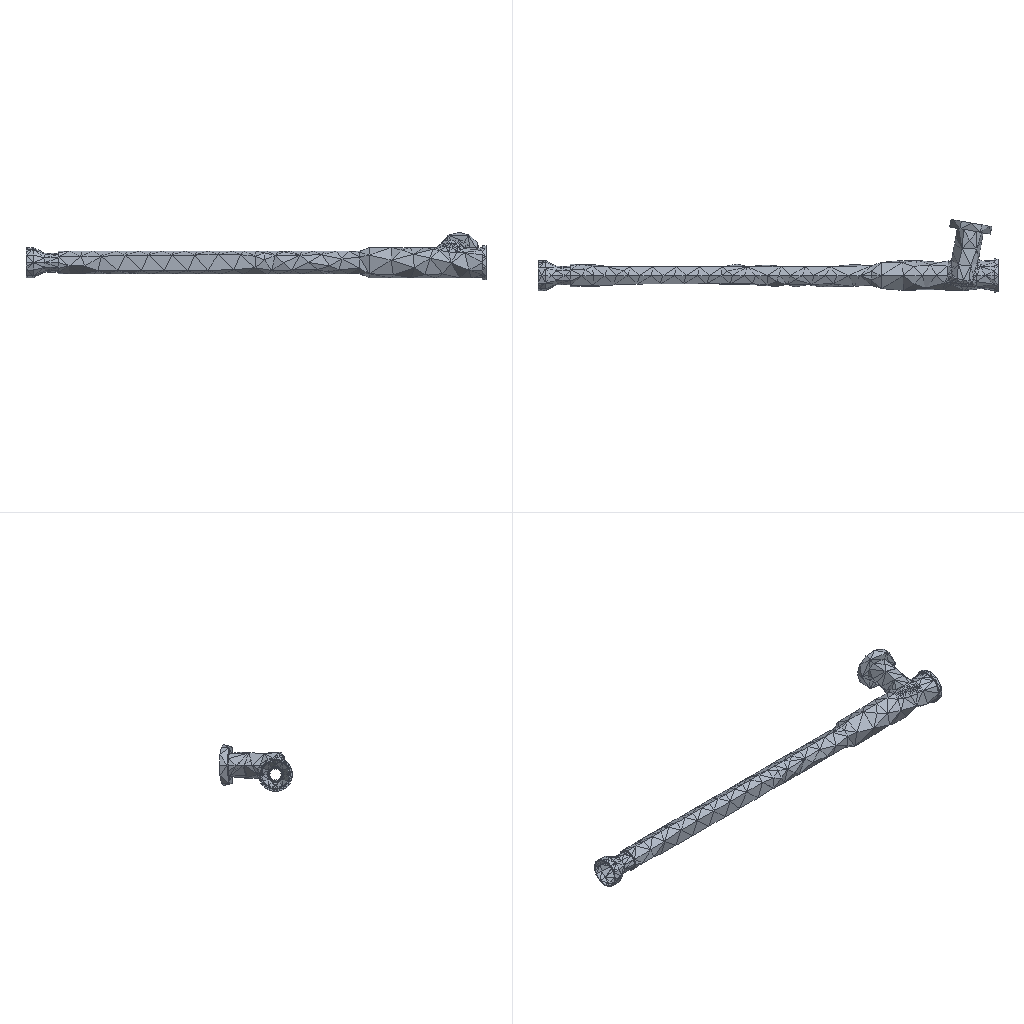Simulation study | ansys workbench
Ansys APDL input file, long lists of numbers shortened:
/batch
/config,noeldb,1     ! force off writing results to database
*get,_wallstrt,active,,time,wall
! ANSYS input file written by Workbench version 2022 R1
! File used for geometry attach: F:\ansys（分析文件汇总)\ansys转向器有限元分析\转向器\分析\动力缸体.STEP
/title,wbnew--____ (H5)
! ****** Begin Custom Load Command Snippet ******
/COM, ACT Extensions:
/COM,     LSDYNA, 2021.1
/COM,
! ****** End   Custom Load Command Snippet ******
*DIM,_wb_ProjectScratch_dir,string,248
_wb_ProjectScratch_dir(1) = 'C:\Users\Administrator\AppData\Local\Temp\WB_Administrator_18756_2\_ProjectScratch\Scr1D13\'
*DIM,_wb_SolverFiles_dir,string,248
_wb_SolverFiles_dir(1) = 'C:\Users\Administrator\AppData\Local\Temp\WB_Administrator_18756_2\wbnew_files\dp0\SYS-2\MECH\'
*DIM,_wb_userfiles_dir,string,248
_wb_userfiles_dir(1) = 'C:\Users\Administrator\AppData\Local\Temp\WB_Administrator_18756_2\wbnew_files\user_files\'
/com,--- Data in consistent NMM units. See Solving Units in the help system for more information.
/units,MPA
/nopr
/wb,file,start              !  signify a WB generated input file
/prep7
! Turn off shape checking because checks already performed inside WB mesher.
! See help system for more information.
SHPP,OFF,,NOWARN
/nolist
etcon,set             ! allow ANSYS to choose best KEYOP's for 180x elements, resets any applicable keyopt to MAPDL defaults
/com,*********** Nodes for the whole assembly ***********
nblock,3,,6333
(1i9,3e20.9e3)
        1     1.131045544E+03     1.243062133E+02     2.500000000E+01
! (5757 more lines like these left out)
-1
/com,*********** Nodes for all Remote Points ***********
nblock,3
(1i9,3e20.9e3)
     5759     5.129297390E+02    -6.539197075E-02    -1.374617690E-01
-1
/wb,elem,start            !  set before creation of elements
/com,*********** Elements for Body 1 "____-FreeParts|NONE" ***********
et,1,187
eblock,19,solid,,2984
(19i9)
        1        1        1        1        0        0        0        0       10        0        1      414      905      670      903     4127     5046     4124     4126
! (5967 more lines like these left out)
-1
/wb,elem,end               !  done creating elements
/com,*********** Send User Defined Coordinate System(s) ***********
csys,0
toffst,273.15,  ! Temperature offset from absolute zero
/com,*********** Set Reference Temperature ***********
tref,22.
/wb,mat,start              !  starting to send materials
/com,*********** Send Materials ***********
Temperature = 'TEMP' ! Temperature
MP,DENS,1,7.85e-09,	! tonne mm^-3
MP,ALPX,1,1.2e-05,	! C^-1
MP,C,1,434000000,	! mm^2 s^-2 C^-1
MP,KXX,1,60.5,	! tonne mm s^-3 C^-1
MP,RSVX,1,0.00017,	! ohm mm
MP,EX,1,200000,	! tonne s^-2 mm^-1
MP,NUXY,1,0.3,
MP,MURX,1,10000,
/wb,mat,end                !  done sending materials
!************************* Model Summary ********************
!____-FreeParts|NONE,	结构钢,	matid,	1
!************************* End Model Summary ********************
! get the diagonal of the bounding box. Needed later for other things
*get,_xmin,node,,mnloc,x
*get,_ymin,node,,mnloc,y
*get,_zmin,node,,mnloc,z
*get,_xmax,node,,mxloc,x
*get,_ymax,node,,mxloc,y
*get,_zmax,node,,mxloc,z
_ASMDIAG=(_xmax-_xmin)*(_xmax-_xmin)+(_ymax-_ymin)*(_ymax-_ymin)+(_zmax-_zmin)*(_zmax-_zmin)
_ASMDIAG=SQRT(_ASMDIAG)
/wb,contact,start          !  starting to send contact
/wb,contact,end            !  done creating contacts
/golist
/wb,load,start             !  starting to send loads
/com,*********** Fixed Supports ***********
CMBLOCK,_FIXEDSU,NODE,      298
(8i10)
        69        70        71        72        73        74        75        76
! (37 more lines like these left out)
cmsel,s,_FIXEDSU
d,all,all
nsel,all
/com,*********** Create Remote Point "内部远程点" ***********
! -------- Remote Point Used by "力矩" --------
*set,tid,3
*set,cid,2
et,cid,174
et,tid,170
keyo,tid,2,1               ! Don't fix the pilot node
keyo,tid,4,111111
keyo,cid,12,5              ! Bonded Contact
keyo,cid,4,1               ! Deformable RBE3 style load
keyo,cid,2,2               ! MPC style contact
eblock,10,,,616
(15i9)
     4772        2        2        2        0       92      415      433      433     1671     4128      433     1672
! (615 more lines like these left out)
-1
*set,_npilot,5759
_npilot32=_npilot
type,tid
mat ,cid
real,cid
tshape,pilo
en,5388,_npilot
tshape
/com,*********** Construct Moment Using Remote Attachment ***********
/gst,on,on
fini
*get,_numnode,node,0,count
*get,_numelem,elem,0,count
*get, _MAXELEMNUM, elem, 0, NUM, MAX
*get, _MAXNODENUM, node, 0, NUM, MAX
*get, _MAXELEMTYPE, etyp, 0, NUM, MAX
*get, _MAXREALCONST, real, 0, NUM, MAX
/go
/wb,load,end               !  done creating loads
/com,--- Number of total nodes = %_numnode%
/com,--- Number of contact elements = 616
/com,--- Number of spring elements = 0
/com,--- Number of bearing elements = 0
/com,--- Number of solid elements = 2984
/com,--- Number of condensed parts = 0
/com,--- Number of total elements = %_numelem%
*get,_wallbsol,active,,time,wall
/com,****************************************************************************
/com,*************************    SOLUTION       ********************************
/com,****************************************************************************
/solu
antype,0                   ! static analysis
_thickRatio=  0     ! Ratio of thick parts in the model
eqsl,sparse,,,,,1
cntr,print,1               ! print out contact info and also make no initial contact an error
dmpoption,emat,no             ! Don't combine emat file for DANSYS
dmpoption,esav,no             ! Don't combine esav file for DANSYS
nldiag,cont,iter           ! print out contact info each equilibrium iteration
rescontrol,,none                 ! Do not keep any restart files
/com,****************************************************
/com,******************* SOLVE FOR LS 1 OF 1 ****************
nsel,s,node,,5759
f,all,mx,5000000.
f,all,my,0.
f,all,mz,0.
nsel,all
/nopr
/gopr
nsub,1,1,1
time,1.
outres,erase
outres,all,none
outres,nsol,all,
outres,rsol,all
outres,eangl,all
outres,etmp,all
outres,veng,all
outres,strs,all,
outres,epel,all,
outres,eppl,all,
outres,cont,all,
! *********** WB SOLVE COMMAND ***********
! check interactive state
*get,ANSINTER_,active,,int
*if,ANSINTER_,ne,0,then
/eof
*endif
solve
/com *************** Write FE CONNECTORS *********
CEWRITE,file,ce,,INTE
/com,****************************************************
/com,*************** FINISHED SOLVE FOR LS 1 *************
*get,_wallasol,active,,time,wall
/nopr
*get,_numnode,node,0,count
*get,_numelem,elem,0,count
*get, _MAXELEMNUM, elem, 0, NUM, MAX
*get, _MAXNODENUM, node, 0, NUM, MAX,,,INTERNAL
*get, _MAXELEMTYPE, etyp, 0, NUM, MAX
*get, _MAXREALCONST, real, 0, NUM, MAX
/gopr
/post1
xmlo,ENCODING,ISO-8859-1
xmlo,parm
/xml,parm,xml
fini
/gopr
*get,_walldone,active,,time,wall
_preptime=(_wallbsol-_wallstrt)*3600
_solvtime=(_wallasol-_wallbsol)*3600
_posttime=(_walldone-_wallasol)*3600
_totaltim=(_walldone-_wallstrt)*3600
*get,_dlbratio,active,0,solu,dlbr
*get,_combtime,active,0,solu,comb
*get,_ssmode,active,0,solu,ssmm
*get,_ndofs,active,0,solu,ndof
*get,_sol_end_time,active,0,set,time
*if,_sol_end_time,eq,1.,then
/fclean				!clean distributed files
*endif
/com,--- Total number of nodes = %_numnode%
/com,--- Total number of elements = %_numelem%
/com,--- Element load balance ratio = %_dlbratio%
/com,--- Time to combine distributed files = %_combtime%
/com,--- Sparse memory mode = %_ssmode%
/com,--- Number of DOF = %_ndofs%
/wb,file,end               ! done with WB generated input